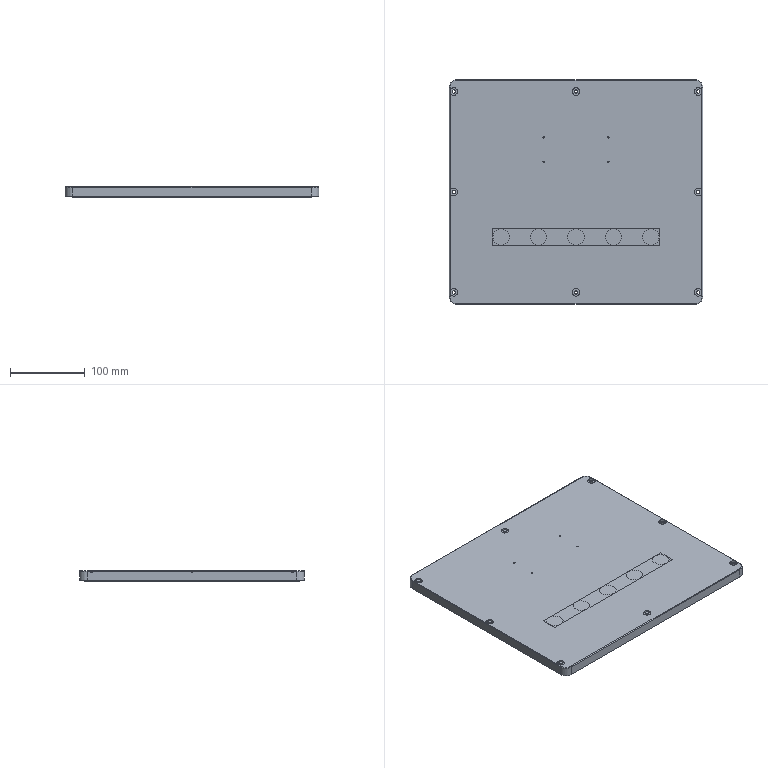NC program | NX | posted with a generic post | part box 338 x 300 x 14.5 mm
Lines 2602 to 2756 of 2756:
(ZLEVEL_PROFILE_2_COPY , TOOL : D4A45)
N5136 T21 M6
N5138 G54
N5140 G17 G0 G90 X161.821 Y0.39 S9500 M3
N5142 G43 Z30. H21
N5144 Z-1.
N5146 G94 G1 Z-2.5 F1250.
N5148 X161.246 Y-0.658
N5150 G3 X161.254 Y-1.058 R0.4
N5152 X161.255 Y1.059 R-2.041
N5154 X161.246 Y0.659 R0.4
N5156 G1 X161.821 Y-0.389
N5158 Z-1.
N5160 G0 Z30.
N5162 X163.806 Y-134.944
N5164 Z-1.
N5166 G1 Z-2.5
N5168 X164.841 Y-134.346
N5170 G3 X165.041 Y-134. R0.4
N5172 X163. Y-131.959 R2.041
N5174 X165.041 Y-134. R-2.041
N5176 X164.841 Y-133.654 R0.4
N5178 G1 X163.806 Y-133.056
N5180 Z-1.
N5182 G0 Z30.
N5184 X-163.806
N5186 Z-1.
N5188 G1 Z-2.5
N5190 X-164.841 Y-133.654
N5192 G3 X-165.041 Y-134. R0.4
N5194 X-163. Y-136.041 R2.041
N5196 X-165.041 Y-134. R-2.041
N5198 X-164.841 Y-134.346 R0.4
N5200 G1 X-163.806 Y-134.944
N5202 Z-1.
N5204 G0 Z30.
N5206 X-0.693 Y-137.241
N5208 Z-1.
N5210 G1 Z-2.5
N5212 X-0.346 Y-137.841
N5214 G3 X0. Y-138.041 R0.4
N5216 G1 X144.
N5218 G3 X153.041 Y-129. R9.041
N5220 G1 Y129.
N5222 G3 X144. Y138.041 R9.041
N5224 G1 X-144.
N5226 G3 X-153.041 Y129. R9.041
N5228 G1 Y-129.
N5230 G3 X-144. Y-138.041 R9.041
N5232 G1 X0.
N5234 G3 X0.346 Y-137.841 R0.4
N5236 G1 X0.693 Y-137.241
N5238 Z-1.
N5240 G0 Z30.
N5242 X163.806 Y133.056
N5244 Z-1.
N5246 G1 Z-2.5
N5248 X164.841 Y133.654
N5250 G3 X165.041 Y134. R0.4
N5252 X163. Y136.041 R2.041
N5254 X165.041 Y134. R-2.041
N5256 X164.841 Y134.346 R0.4
N5258 G1 X163.806 Y134.944
N5260 Z-1.
N5262 G0 Z30.
N5264 X-163.806
N5266 Z-1.
N5268 G1 Z-2.5
N5270 X-164.841 Y134.346
N5272 G3 X-165.041 Y134. R0.4
N5274 X-163. Y131.959 R2.041
N5276 X-165.041 Y134. R-2.041
N5278 X-164.841 Y133.654 R0.4
N5280 G1 X-163.806 Y133.056
N5282 Z-1.
N5284 G0 Z30.
N5286 X-161.822 Y-0.392
N5288 Z-1.
N5290 G1 Z-2.5
N5292 X-161.245 Y0.655
N5294 G3 X-161.253 Y1.055 R0.4
N5296 X-161.251 Y-1.053 R-2.041
N5298 X-161.244 Y-0.654 R0.4
N5300 G1 X-161.822 Y0.393
N5302 Z-1.
N5304 G0 Z30.
N5306 X-0.693 Y151.759
N5308 Z-1.
N5310 G1 Z-2.5
N5312 X-0.346 Y151.159
N5314 G3 X0. Y150.959 R0.4
N5316 G1 X159.
N5318 G2 X169.959 Y140. R10.959
N5320 G1 Y-140.
N5322 G2 X159. Y-150.959 R10.959
N5324 G1 X-159.
N5326 G2 X-169.959 Y-140. R10.959
N5328 G1 Y140.
N5330 G2 X-159. Y150.959 R10.959
N5332 G1 X0.
N5334 G3 X0.346 Y151.159 R0.4
N5336 G1 X0.693 Y151.759
N5338 Z-1.
N5340 G0 Z30.
N5342 M5
(刀补14 , TOOL : D10JING)
N5344 T14 M6
N5346 G54
N5348 G17 G0 G90 X-146.499 Y150.394 S9500 M3
N5350 G43 Z30. H14
N5352 Z0.
N5354 G94 G1 Z-1.5 F1000.
N5356 G41 X-146.465 Y150.3 D14
N5358 X-145.916 Y149.35
N5360 G3 X-145.05 Y148.85 R1.
N5362 G1 X145.05 F1200.
N5364 G2 X163.75 Y130.15 R18.7
N5366 G1 Y-130.15
N5368 G2 X145.05 Y-148.85 R18.7
N5370 G1 X-145.05
N5372 G2 X-163.75 Y-130.15 R18.7
N5374 G1 Y130.15
N5376 G2 X-145.05 Y148.85 R18.7
N5378 G3 X-144.184 Y149.35 R1.
N5380 G1 X-143.607 Y150.35
N5382 G40
N5384 X-143.572 Y150.444
N5386 Z0.
N5388 G0 Z30.
N5390 X146.661 Y135.325
N5392 Z0.
N5394 G1 Z-1.5 F1000.
N5396 G41 X146.627 Y135.419
N5398 X145.916 Y136.65
N5400 G3 X145.05 Y137.15 R1.
N5402 G1 X-145.05 F1200.
N5404 G3 X-152.05 Y130.15 R7.
N5406 G1 Y-130.15
N5408 G3 X-145.05 Y-137.15 R7.
N5410 G1 X145.05
N5412 G3 X152.05 Y-130.15 R7.
N5414 G1 Y130.15
N5416 G3 X145.05 Y137.15 R7.
N5418 X144.184 Y136.65 R1.
N5420 G1 X143.607 Y135.65
N5422 G40
N5424 X143.572 Y135.556
N5426 Z0.
N5428 G0 Z30.
N5430 M5
N5432 M2